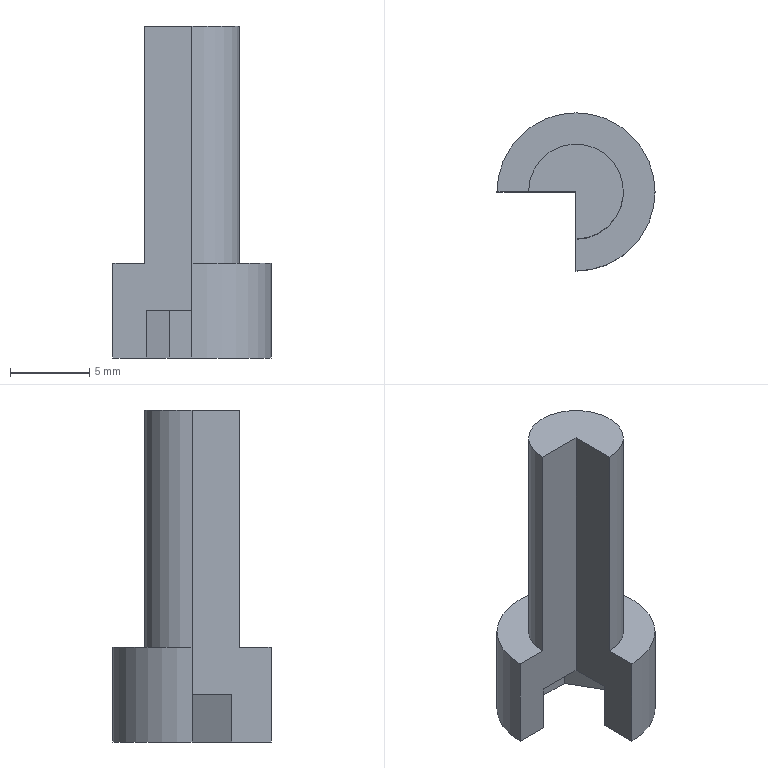Part | STEP file | LG M6_1.5F | 1 solid | 14 faces | box 10 x 10 x 21 mm | volume 622.411 mm3 | plane 11 | cylinder 3 | commonest cylinder face diameters 10 x2 6 x1
STEP:
#1=CARTESIAN_POINT('',(0.,0.,0.));
#2=DIRECTION('',(0.,0.,1.));
#3=DIRECTION('',(1.,0.,0.));
#4=AXIS2_PLACEMENT_3D('',#1,#2,#3);
#5=CARTESIAN_POINT('',(0.,-5.,-6.));
#6=VERTEX_POINT('',#5);
#7=CARTESIAN_POINT('',(5.,0.,-6.));
#8=VERTEX_POINT('',#7);
#9=CARTESIAN_POINT('',(0.,0.,-6.));
#10=DIRECTION('',(0.,0.,1.));
#11=DIRECTION('',(1.,0.,0.));
#12=AXIS2_PLACEMENT_3D('',#9,#10,#11);
#13=CIRCLE('',#12,5.);
#14=CARTESIAN_POINT('',(0.,0.,-6.));
#15=DIRECTION('',(0.,0.,1.));
#16=DIRECTION('',(1.,0.,0.));
#17=AXIS2_PLACEMENT_3D('',#14,#15,#16);
#18=CYLINDRICAL_SURFACE('',#17,5.);
#19=CARTESIAN_POINT('',(0.,0.));
#20=DIRECTION('',(1.,0.));
#21=VECTOR('',#20,1.);
#22=LINE('',#19,#21);
#23=(GEOMETRIC_REPRESENTATION_CONTEXT(2)PARAMETRIC_REPRESENTATION_CONTEXT()REPRESENTATION_CONTEXT('',''));
#24=DEFINITIONAL_REPRESENTATION('',(#22),#23);
#25=PCURVE('',#18,#24);
#26=CARTESIAN_POINT('',(0.,0.,-6.));
#27=DIRECTION('',(0.,0.,1.));
#28=DIRECTION('',(1.,0.,0.));
#29=AXIS2_PLACEMENT_3D('',#26,#27,#28);
#30=PLANE('',#29);
#31=CARTESIAN_POINT('',(0.,0.));
#32=DIRECTION('',(1.,0.));
#33=AXIS2_PLACEMENT_2D('',#31,#32);
#34=CIRCLE('',#33,5.);
#35=(GEOMETRIC_REPRESENTATION_CONTEXT(2)PARAMETRIC_REPRESENTATION_CONTEXT()REPRESENTATION_CONTEXT('',''));
#36=DEFINITIONAL_REPRESENTATION('',(#34),#35);
#37=PCURVE('',#30,#36);
#38=SURFACE_CURVE('',#13,(#25,#37),.PCURVE_S1.);
#39=EDGE_CURVE('',#6,#8,#38,.T.);
#40=ORIENTED_EDGE('',*,*,#39,.T.);
#41=CARTESIAN_POINT('',(5.,0.,0.));
#42=VERTEX_POINT('',#41);
#43=CARTESIAN_POINT('',(5.,0.,-6.));
#44=DIRECTION('',(0.,0.,1.));
#45=VECTOR('',#44,1.);
#46=LINE('',#43,#45);
#47=CARTESIAN_POINT('',(6.283,0.));
#48=DIRECTION('',(0.,1.));
#49=VECTOR('',#48,1.);
#50=LINE('',#47,#49);
#51=(GEOMETRIC_REPRESENTATION_CONTEXT(2)PARAMETRIC_REPRESENTATION_CONTEXT()REPRESENTATION_CONTEXT('',''));
#52=DEFINITIONAL_REPRESENTATION('',(#50),#51);
#53=PCURVE('',#18,#52);
#54=CARTESIAN_POINT('',(0.,0.,-6.));
#55=DIRECTION('',(0.,0.,1.));
#56=DIRECTION('',(1.,0.,0.));
#57=AXIS2_PLACEMENT_3D('',#54,#55,#56);
#58=CYLINDRICAL_SURFACE('',#57,5.);
#59=CARTESIAN_POINT('',(0.,0.));
#60=DIRECTION('',(0.,1.));
#61=VECTOR('',#60,1.);
#62=LINE('',#59,#61);
#63=(GEOMETRIC_REPRESENTATION_CONTEXT(2)PARAMETRIC_REPRESENTATION_CONTEXT()REPRESENTATION_CONTEXT('',''));
#64=DEFINITIONAL_REPRESENTATION('',(#62),#63);
#65=PCURVE('',#58,#64);
#66=SURFACE_CURVE('',#46,(#53,#65),.PCURVE_S1.);
#67=EDGE_CURVE('',#8,#42,#66,.T.);
#68=ORIENTED_EDGE('',*,*,#67,.T.);
#69=CARTESIAN_POINT('',(0.,-5.,0.));
#70=VERTEX_POINT('',#69);
#71=CARTESIAN_POINT('',(0.,0.,0.));
#72=DIRECTION('',(0.,0.,1.));
#73=DIRECTION('',(1.,0.,0.));
#74=AXIS2_PLACEMENT_3D('',#71,#72,#73);
#75=CIRCLE('',#74,5.);
#76=CARTESIAN_POINT('',(0.,6.));
#77=DIRECTION('',(1.,0.));
#78=VECTOR('',#77,1.);
#79=LINE('',#76,#78);
#80=(GEOMETRIC_REPRESENTATION_CONTEXT(2)PARAMETRIC_REPRESENTATION_CONTEXT()REPRESENTATION_CONTEXT('',''));
#81=DEFINITIONAL_REPRESENTATION('',(#79),#80);
#82=PCURVE('',#18,#81);
#83=CARTESIAN_POINT('',(0.,0.,0.));
#84=DIRECTION('',(0.,0.,1.));
#85=DIRECTION('',(1.,0.,0.));
#86=AXIS2_PLACEMENT_3D('',#83,#84,#85);
#87=PLANE('',#86);
#88=CARTESIAN_POINT('',(0.,0.));
#89=DIRECTION('',(1.,0.));
#90=AXIS2_PLACEMENT_2D('',#88,#89);
#91=CIRCLE('',#90,5.);
#92=(GEOMETRIC_REPRESENTATION_CONTEXT(2)PARAMETRIC_REPRESENTATION_CONTEXT()REPRESENTATION_CONTEXT('',''));
#93=DEFINITIONAL_REPRESENTATION('',(#91),#92);
#94=PCURVE('',#87,#93);
#95=SURFACE_CURVE('',#75,(#82,#94),.PCURVE_S1.);
#96=EDGE_CURVE('',#70,#42,#95,.T.);
#97=ORIENTED_EDGE('',*,*,#96,.F.);
#98=CARTESIAN_POINT('',(0.,-5.,-6.));
#99=DIRECTION('',(0.,0.,-1.));
#100=VECTOR('',#99,1.);
#101=LINE('',#98,#100);
#102=CARTESIAN_POINT('',(4.712,0.));
#103=DIRECTION('',(0.,-1.));
#104=VECTOR('',#103,1.);
#105=LINE('',#102,#104);
#106=(GEOMETRIC_REPRESENTATION_CONTEXT(2)PARAMETRIC_REPRESENTATION_CONTEXT()REPRESENTATION_CONTEXT('',''));
#107=DEFINITIONAL_REPRESENTATION('',(#105),#106);
#108=PCURVE('',#18,#107);
#109=CARTESIAN_POINT('',(0.,33.935,109.834));
#110=DIRECTION('',(-1.,0.,0.));
#111=DIRECTION('',(0.,1.,0.));
#112=AXIS2_PLACEMENT_3D('',#109,#110,#111);
#113=PLANE('',#112);
#114=CARTESIAN_POINT('',(-38.935,115.834));
#115=DIRECTION('',(0.,1.));
#116=VECTOR('',#115,1.);
#117=LINE('',#114,#116);
#118=(GEOMETRIC_REPRESENTATION_CONTEXT(2)PARAMETRIC_REPRESENTATION_CONTEXT()REPRESENTATION_CONTEXT('',''));
#119=DEFINITIONAL_REPRESENTATION('',(#117),#118);
#120=PCURVE('',#113,#119);
#121=SURFACE_CURVE('',#101,(#108,#120),.PCURVE_S1.);
#122=EDGE_CURVE('',#70,#6,#121,.T.);
#123=ORIENTED_EDGE('',*,*,#122,.T.);
#124=EDGE_LOOP('',(#40,#68,#97,#123));
#125=FACE_BOUND('',#124,.T.);
#126=ADVANCED_FACE('',(#125),#18,.T.);
#127=CARTESIAN_POINT('',(0.,-2.51,-3.));
#128=VERTEX_POINT('',#127);
#129=CARTESIAN_POINT('',(0.,-2.51,-6.));
#130=VERTEX_POINT('',#129);
#131=CARTESIAN_POINT('',(0.,-2.51,-3.));
#132=DIRECTION('',(0.,0.,-1.));
#133=VECTOR('',#132,1.);
#134=LINE('',#131,#133);
#135=CARTESIAN_POINT('',(1.449,-2.51,-3.));
#136=DIRECTION('',(0.,-1.,0.));
#137=DIRECTION('',(0.,0.,-1.));
#138=AXIS2_PLACEMENT_3D('',#135,#136,#137);
#139=PLANE('',#138);
#140=CARTESIAN_POINT('',(0.,-1.449));
#141=DIRECTION('',(1.,0.));
#142=VECTOR('',#141,1.);
#143=LINE('',#140,#142);
#144=(GEOMETRIC_REPRESENTATION_CONTEXT(2)PARAMETRIC_REPRESENTATION_CONTEXT()REPRESENTATION_CONTEXT('',''));
#145=DEFINITIONAL_REPRESENTATION('',(#143),#144);
#146=PCURVE('',#139,#145);
#147=CARTESIAN_POINT('',(-36.445,112.834));
#148=DIRECTION('',(0.,1.));
#149=VECTOR('',#148,1.);
#150=LINE('',#147,#149);
#151=(GEOMETRIC_REPRESENTATION_CONTEXT(2)PARAMETRIC_REPRESENTATION_CONTEXT()REPRESENTATION_CONTEXT('',''));
#152=DEFINITIONAL_REPRESENTATION('',(#150),#151);
#153=PCURVE('',#113,#152);
#154=SURFACE_CURVE('',#134,(#146,#153),.PCURVE_S1.);
#155=EDGE_CURVE('',#128,#130,#154,.T.);
#156=ORIENTED_EDGE('',*,*,#155,.F.);
#157=CARTESIAN_POINT('',(1.449,-2.51,-3.));
#158=VERTEX_POINT('',#157);
#159=CARTESIAN_POINT('',(1.449,-2.51,-3.));
#160=DIRECTION('',(-1.,0.,0.));
#161=VECTOR('',#160,1.);
#162=LINE('',#159,#161);
#163=CARTESIAN_POINT('',(0.,0.));
#164=DIRECTION('',(0.,-1.));
#165=VECTOR('',#164,1.);
#166=LINE('',#163,#165);
#167=(GEOMETRIC_REPRESENTATION_CONTEXT(2)PARAMETRIC_REPRESENTATION_CONTEXT()REPRESENTATION_CONTEXT('',''));
#168=DEFINITIONAL_REPRESENTATION('',(#166),#167);
#169=PCURVE('',#139,#168);
#170=CARTESIAN_POINT('',(0.,0.,-3.));
#171=DIRECTION('',(0.,0.,-1.));
#172=DIRECTION('',(-1.,0.,0.));
#173=AXIS2_PLACEMENT_3D('',#170,#171,#172);
#174=PLANE('',#173);
#175=CARTESIAN_POINT('',(-1.449,-2.51));
#176=DIRECTION('',(1.,0.));
#177=VECTOR('',#176,1.);
#178=LINE('',#175,#177);
#179=(GEOMETRIC_REPRESENTATION_CONTEXT(2)PARAMETRIC_REPRESENTATION_CONTEXT()REPRESENTATION_CONTEXT('',''));
#180=DEFINITIONAL_REPRESENTATION('',(#178),#179);
#181=PCURVE('',#174,#180);
#182=SURFACE_CURVE('',#162,(#169,#181),.PCURVE_S1.);
#183=EDGE_CURVE('',#158,#128,#182,.T.);
#184=ORIENTED_EDGE('',*,*,#183,.F.);
#185=CARTESIAN_POINT('',(1.449,-2.51,-6.));
#186=VERTEX_POINT('',#185);
#187=CARTESIAN_POINT('',(1.449,-2.51,-3.));
#188=DIRECTION('',(0.,0.,-1.));
#189=VECTOR('',#188,1.);
#190=LINE('',#187,#189);
#191=CARTESIAN_POINT('',(0.,0.));
#192=DIRECTION('',(1.,0.));
#193=VECTOR('',#192,1.);
#194=LINE('',#191,#193);
#195=(GEOMETRIC_REPRESENTATION_CONTEXT(2)PARAMETRIC_REPRESENTATION_CONTEXT()REPRESENTATION_CONTEXT('',''));
#196=DEFINITIONAL_REPRESENTATION('',(#194),#195);
#197=PCURVE('',#139,#196);
#198=CARTESIAN_POINT('',(2.898,0.,-3.));
#199=DIRECTION('',(0.866,-0.5,0.));
#200=DIRECTION('',(0.5,0.866,0.));
#201=AXIS2_PLACEMENT_3D('',#198,#199,#200);
#202=PLANE('',#201);
#203=CARTESIAN_POINT('',(-2.898,0.));
#204=DIRECTION('',(0.,-1.));
#205=VECTOR('',#204,1.);
#206=LINE('',#203,#205);
#207=(GEOMETRIC_REPRESENTATION_CONTEXT(2)PARAMETRIC_REPRESENTATION_CONTEXT()REPRESENTATION_CONTEXT('',''));
#208=DEFINITIONAL_REPRESENTATION('',(#206),#207);
#209=PCURVE('',#202,#208);
#210=SURFACE_CURVE('',#190,(#197,#209),.PCURVE_S1.);
#211=EDGE_CURVE('',#158,#186,#210,.T.);
#212=ORIENTED_EDGE('',*,*,#211,.T.);
#213=CARTESIAN_POINT('',(1.449,-2.51,-6.));
#214=DIRECTION('',(-1.,0.,0.));
#215=VECTOR('',#214,1.);
#216=LINE('',#213,#215);
#217=CARTESIAN_POINT('',(3.,0.));
#218=DIRECTION('',(0.,-1.));
#219=VECTOR('',#218,1.);
#220=LINE('',#217,#219);
#221=(GEOMETRIC_REPRESENTATION_CONTEXT(2)PARAMETRIC_REPRESENTATION_CONTEXT()REPRESENTATION_CONTEXT('',''));
#222=DEFINITIONAL_REPRESENTATION('',(#220),#221);
#223=PCURVE('',#139,#222);
#224=CARTESIAN_POINT('',(1.449,-2.51));
#225=DIRECTION('',(-1.,0.));
#226=VECTOR('',#225,1.);
#227=LINE('',#224,#226);
#228=(GEOMETRIC_REPRESENTATION_CONTEXT(2)PARAMETRIC_REPRESENTATION_CONTEXT()REPRESENTATION_CONTEXT('',''));
#229=DEFINITIONAL_REPRESENTATION('',(#227),#228);
#230=PCURVE('',#30,#229);
#231=SURFACE_CURVE('',#216,(#223,#230),.PCURVE_S1.);
#232=EDGE_CURVE('',#186,#130,#231,.T.);
#233=ORIENTED_EDGE('',*,*,#232,.T.);
#234=EDGE_LOOP('',(#156,#184,#212,#233));
#235=FACE_BOUND('',#234,.T.);
#236=ADVANCED_FACE('',(#235),#139,.F.);
#237=CARTESIAN_POINT('',(-3.,0.,0.));
#238=VERTEX_POINT('',#237);
#239=CARTESIAN_POINT('',(-5.,0.,0.));
#240=VERTEX_POINT('',#239);
#241=CARTESIAN_POINT('',(0.,0.,0.));
#242=DIRECTION('',(-1.,0.,0.));
#243=VECTOR('',#242,1.);
#244=LINE('',#241,#243);
#245=CARTESIAN_POINT('',(0.,0.));
#246=DIRECTION('',(-1.,0.));
#247=VECTOR('',#246,1.);
#248=LINE('',#245,#247);
#249=(GEOMETRIC_REPRESENTATION_CONTEXT(2)PARAMETRIC_REPRESENTATION_CONTEXT()REPRESENTATION_CONTEXT('',''));
#250=DEFINITIONAL_REPRESENTATION('',(#248),#249);
#251=PCURVE('',#87,#250);
#252=CARTESIAN_POINT('',(0.,0.,98.57));
#253=DIRECTION('',(0.,1.,0.));
#254=DIRECTION('',(1.,0.,0.));
#255=AXIS2_PLACEMENT_3D('',#252,#253,#254);
#256=PLANE('',#255);
#257=CARTESIAN_POINT('',(0.,98.57));
#258=DIRECTION('',(-1.,0.));
#259=VECTOR('',#258,1.);
#260=LINE('',#257,#259);
#261=(GEOMETRIC_REPRESENTATION_CONTEXT(2)PARAMETRIC_REPRESENTATION_CONTEXT()REPRESENTATION_CONTEXT('',''));
#262=DEFINITIONAL_REPRESENTATION('',(#260),#261);
#263=PCURVE('',#256,#262);
#264=SURFACE_CURVE('',#244,(#251,#263),.PCURVE_S1.);
#265=EDGE_CURVE('',#238,#240,#264,.T.);
#266=ORIENTED_EDGE('',*,*,#265,.F.);
#267=CARTESIAN_POINT('',(0.,-3.,0.));
#268=VERTEX_POINT('',#267);
#269=CARTESIAN_POINT('',(0.,0.,0.));
#270=DIRECTION('',(0.,0.,1.));
#271=DIRECTION('',(1.,0.,0.));
#272=AXIS2_PLACEMENT_3D('',#269,#270,#271);
#273=CIRCLE('',#272,3.);
#274=CARTESIAN_POINT('',(0.,0.));
#275=DIRECTION('',(1.,0.));
#276=AXIS2_PLACEMENT_2D('',#274,#275);
#277=CIRCLE('',#276,3.);
#278=(GEOMETRIC_REPRESENTATION_CONTEXT(2)PARAMETRIC_REPRESENTATION_CONTEXT()REPRESENTATION_CONTEXT('',''));
#279=DEFINITIONAL_REPRESENTATION('',(#277),#278);
#280=PCURVE('',#87,#279);
#281=CARTESIAN_POINT('',(0.,0.,15.));
#282=DIRECTION('',(0.,0.,-1.));
#283=DIRECTION('',(-1.,0.,0.));
#284=AXIS2_PLACEMENT_3D('',#281,#282,#283);
#285=CYLINDRICAL_SURFACE('',#284,3.);
#286=CARTESIAN_POINT('',(9.425,15.));
#287=DIRECTION('',(-1.,0.));
#288=VECTOR('',#287,1.);
#289=LINE('',#286,#288);
#290=(GEOMETRIC_REPRESENTATION_CONTEXT(2)PARAMETRIC_REPRESENTATION_CONTEXT()REPRESENTATION_CONTEXT('',''));
#291=DEFINITIONAL_REPRESENTATION('',(#289),#290);
#292=PCURVE('',#285,#291);
#293=SURFACE_CURVE('',#273,(#280,#292),.PCURVE_S1.);
#294=EDGE_CURVE('',#268,#238,#293,.T.);
#295=ORIENTED_EDGE('',*,*,#294,.F.);
#296=CARTESIAN_POINT('',(0.,0.,0.));
#297=DIRECTION('',(0.,-1.,0.));
#298=VECTOR('',#297,1.);
#299=LINE('',#296,#298);
#300=CARTESIAN_POINT('',(0.,0.));
#301=DIRECTION('',(0.,-1.));
#302=VECTOR('',#301,1.);
#303=LINE('',#300,#302);
#304=(GEOMETRIC_REPRESENTATION_CONTEXT(2)PARAMETRIC_REPRESENTATION_CONTEXT()REPRESENTATION_CONTEXT('',''));
#305=DEFINITIONAL_REPRESENTATION('',(#303),#304);
#306=PCURVE('',#87,#305);
#307=CARTESIAN_POINT('',(-33.935,109.834));
#308=DIRECTION('',(-1.,0.));
#309=VECTOR('',#308,1.);
#310=LINE('',#307,#309);
#311=(GEOMETRIC_REPRESENTATION_CONTEXT(2)PARAMETRIC_REPRESENTATION_CONTEXT()REPRESENTATION_CONTEXT('',''));
#312=DEFINITIONAL_REPRESENTATION('',(#310),#311);
#313=PCURVE('',#113,#312);
#314=SURFACE_CURVE('',#299,(#306,#313),.PCURVE_S1.);
#315=EDGE_CURVE('',#268,#70,#314,.T.);
#316=ORIENTED_EDGE('',*,*,#315,.T.);
#317=ORIENTED_EDGE('',*,*,#96,.T.);
#318=CARTESIAN_POINT('',(0.,0.,0.));
#319=DIRECTION('',(0.,0.,1.));
#320=DIRECTION('',(1.,0.,0.));
#321=AXIS2_PLACEMENT_3D('',#318,#319,#320);
#322=CIRCLE('',#321,5.);
#323=CARTESIAN_POINT('',(0.,0.));
#324=DIRECTION('',(1.,0.));
#325=AXIS2_PLACEMENT_2D('',#323,#324);
#326=CIRCLE('',#325,5.);
#327=(GEOMETRIC_REPRESENTATION_CONTEXT(2)PARAMETRIC_REPRESENTATION_CONTEXT()REPRESENTATION_CONTEXT('',''));
#328=DEFINITIONAL_REPRESENTATION('',(#326),#327);
#329=PCURVE('',#87,#328);
#330=CARTESIAN_POINT('',(0.,6.));
#331=DIRECTION('',(1.,0.));
#332=VECTOR('',#331,1.);
#333=LINE('',#330,#332);
#334=(GEOMETRIC_REPRESENTATION_CONTEXT(2)PARAMETRIC_REPRESENTATION_CONTEXT()REPRESENTATION_CONTEXT('',''));
#335=DEFINITIONAL_REPRESENTATION('',(#333),#334);
#336=PCURVE('',#58,#335);
#337=SURFACE_CURVE('',#322,(#329,#336),.PCURVE_S1.);
#338=EDGE_CURVE('',#42,#240,#337,.T.);
#339=ORIENTED_EDGE('',*,*,#338,.T.);
#340=EDGE_LOOP('',(#266,#295,#316,#317,#339));
#341=FACE_BOUND('',#340,.T.);
#342=ADVANCED_FACE('',(#341),#87,.T.);
#343=ORIENTED_EDGE('',*,*,#67,.F.);
#344=CARTESIAN_POINT('',(-5.,0.,-6.));
#345=VERTEX_POINT('',#344);
#346=CARTESIAN_POINT('',(0.,0.,-6.));
#347=DIRECTION('',(0.,0.,1.));
#348=DIRECTION('',(1.,0.,0.));
#349=AXIS2_PLACEMENT_3D('',#346,#347,#348);
#350=CIRCLE('',#349,5.);
#351=CARTESIAN_POINT('',(0.,0.));
#352=DIRECTION('',(1.,0.));
#353=VECTOR('',#352,1.);
#354=LINE('',#351,#353);
#355=(GEOMETRIC_REPRESENTATION_CONTEXT(2)PARAMETRIC_REPRESENTATION_CONTEXT()REPRESENTATION_CONTEXT('',''));
#356=DEFINITIONAL_REPRESENTATION('',(#354),#355);
#357=PCURVE('',#58,#356);
#358=CARTESIAN_POINT('',(0.,0.));
#359=DIRECTION('',(1.,0.));
#360=AXIS2_PLACEMENT_2D('',#358,#359);
#361=CIRCLE('',#360,5.);
#362=(GEOMETRIC_REPRESENTATION_CONTEXT(2)PARAMETRIC_REPRESENTATION_CONTEXT()REPRESENTATION_CONTEXT('',''));
#363=DEFINITIONAL_REPRESENTATION('',(#361),#362);
#364=PCURVE('',#30,#363);
#365=SURFACE_CURVE('',#350,(#357,#364),.PCURVE_S1.);
#366=EDGE_CURVE('',#8,#345,#365,.T.);
#367=ORIENTED_EDGE('',*,*,#366,.T.);
#368=CARTESIAN_POINT('',(-5.,0.,-6.));
#369=DIRECTION('',(0.,0.,-1.));
#370=VECTOR('',#369,1.);
#371=LINE('',#368,#370);
#372=CARTESIAN_POINT('',(3.142,0.));
#373=DIRECTION('',(0.,-1.));
#374=VECTOR('',#373,1.);
#375=LINE('',#372,#374);
#376=(GEOMETRIC_REPRESENTATION_CONTEXT(2)PARAMETRIC_REPRESENTATION_CONTEXT()REPRESENTATION_CONTEXT('',''));
#377=DEFINITIONAL_REPRESENTATION('',(#375),#376);
#378=PCURVE('',#58,#377);
#379=CARTESIAN_POINT('',(-5.,104.57));
#380=DIRECTION('',(0.,1.));
#381=VECTOR('',#380,1.);
#382=LINE('',#379,#381);
#383=(GEOMETRIC_REPRESENTATION_CONTEXT(2)PARAMETRIC_REPRESENTATION_CONTEXT()REPRESENTATION_CONTEXT('',''));
#384=DEFINITIONAL_REPRESENTATION('',(#382),#383);
#385=PCURVE('',#256,#384);
#386=SURFACE_CURVE('',#371,(#378,#385),.PCURVE_S1.);
#387=EDGE_CURVE('',#240,#345,#386,.T.);
#388=ORIENTED_EDGE('',*,*,#387,.F.);
#389=ORIENTED_EDGE('',*,*,#338,.F.);
#390=EDGE_LOOP('',(#343,#367,#388,#389));
#391=FACE_BOUND('',#390,.T.);
#392=ADVANCED_FACE('',(#391),#58,.T.);
#393=CARTESIAN_POINT('',(-2.898,0.,-6.));
#394=VERTEX_POINT('',#393);
#395=CARTESIAN_POINT('',(-1.449,2.51,-6.));
#396=VERTEX_POINT('',#395);
#397=CARTESIAN_POINT('',(-2.898,0.,-6.));
#398=DIRECTION('',(0.5,0.866,0.));
#399=VECTOR('',#398,1.);
#400=LINE('',#397,#399);
#401=CARTESIAN_POINT('',(-2.898,0.));
#402=DIRECTION('',(0.5,0.866));
#403=VECTOR('',#402,1.);
#404=LINE('',#401,#403);
#405=(GEOMETRIC_REPRESENTATION_CONTEXT(2)PARAMETRIC_REPRESENTATION_CONTEXT()REPRESENTATION_CONTEXT('',''));
#406=DEFINITIONAL_REPRESENTATION('',(#404),#405);
#407=PCURVE('',#30,#406);
#408=CARTESIAN_POINT('',(-2.898,0.,-3.));
#409=DIRECTION('',(-0.866,0.5,0.));
#410=DIRECTION('',(-0.5,-0.866,0.));
#411=AXIS2_PLACEMENT_3D('',#408,#409,#410);
#412=PLANE('',#411);
#413=CARTESIAN_POINT('',(0.,-3.));
#414=DIRECTION('',(-1.,0.));
#415=VECTOR('',#414,1.);
#416=LINE('',#413,#415);
#417=(GEOMETRIC_REPRESENTATION_CONTEXT(2)PARAMETRIC_REPRESENTATION_CONTEXT()REPRESENTATION_CONTEXT('',''));
#418=DEFINITIONAL_REPRESENTATION('',(#416),#417);
#419=PCURVE('',#412,#418);
#420=SURFACE_CURVE('',#400,(#407,#419),.PCURVE_S1.);
#421=EDGE_CURVE('',#394,#396,#420,.T.);
#422=ORIENTED_EDGE('',*,*,#421,.F.);
#423=CARTESIAN_POINT('',(0.,0.,-6.));
#424=DIRECTION('',(-1.,0.,0.));
#425=VECTOR('',#424,1.);
#426=LINE('',#423,#425);
#427=CARTESIAN_POINT('',(0.,0.));
#428=DIRECTION('',(-1.,0.));
#429=VECTOR('',#428,1.);
#430=LINE('',#427,#429);
#431=(GEOMETRIC_REPRESENTATION_CONTEXT(2)PARAMETRIC_REPRESENTATION_CONTEXT()REPRESENTATION_CONTEXT('',''));
#432=DEFINITIONAL_REPRESENTATION('',(#430),#431);
#433=PCURVE('',#30,#432);
#434=CARTESIAN_POINT('',(0.,104.57));
#435=DIRECTION('',(-1.,0.));
#436=VECTOR('',#435,1.);
#437=LINE('',#434,#436);
#438=(GEOMETRIC_REPRESENTATION_CONTEXT(2)PARAMETRIC_REPRESENTATION_CONTEXT()REPRESENTATION_CONTEXT('',''));
#439=DEFINITIONAL_REPRESENTATION('',(#437),#438);
#440=PCURVE('',#256,#439);
#441=SURFACE_CURVE('',#426,(#433,#440),.PCURVE_S1.);
#442=EDGE_CURVE('',#394,#345,#441,.T.);
#443=ORIENTED_EDGE('',*,*,#442,.T.);
#444=ORIENTED_EDGE('',*,*,#366,.F.);
#445=ORIENTED_EDGE('',*,*,#39,.F.);
#446=CARTESIAN_POINT('',(0.,0.,-6.));
#447=DIRECTION('',(0.,-1.,0.));
#448=VECTOR('',#447,1.);
#449=LINE('',#446,#448);
#450=CARTESIAN_POINT('',(0.,0.));
#451=DIRECTION('',(0.,-1.));
#452=VECTOR('',#451,1.);
#453=LINE('',#450,#452);
#454=(GEOMETRIC_REPRESENTATION_CONTEXT(2)PARAMETRIC_REPRESENTATION_CONTEXT()REPRESENTATION_CONTEXT('',''));
#455=DEFINITIONAL_REPRESENTATION('',(#453),#454);
#456=PCURVE('',#30,#455);
#457=CARTESIAN_POINT('',(-33.935,115.834));
#458=DIRECTION('',(-1.,0.));
#459=VECTOR('',#458,1.);
#460=LINE('',#457,#459);
#461=(GEOMETRIC_REPRESENTATION_CONTEXT(2)PARAMETRIC_REPRESENTATION_CONTEXT()REPRESENTATION_CONTEXT('',''));
#462=DEFINITIONAL_REPRESENTATION('',(#460),#461);
#463=PCURVE('',#113,#462);
#464=SURFACE_CURVE('',#449,(#456,#463),.PCURVE_S1.);
#465=EDGE_CURVE('',#130,#6,#464,.T.);
#466=ORIENTED_EDGE('',*,*,#465,.F.);
#467=ORIENTED_EDGE('',*,*,#232,.F.);
#468=CARTESIAN_POINT('',(2.898,0.,-6.));
#469=VERTEX_POINT('',#468);
#470=CARTESIAN_POINT('',(2.898,0.,-6.));
#471=DIRECTION('',(-0.5,-0.866,0.));
#472=VECTOR('',#471,1.);
#473=LINE('',#470,#472);
#474=CARTESIAN_POINT('',(2.898,0.));
#475=DIRECTION('',(-0.5,-0.866));
#476=VECTOR('',#475,1.);
#477=LINE('',#474,#476);
#478=(GEOMETRIC_REPRESENTATION_CONTEXT(2)PARAMETRIC_REPRESENTATION_CONTEXT()REPRESENTATION_CONTEXT('',''));
#479=DEFINITIONAL_REPRESENTATION('',(#477),#478);
#480=PCURVE('',#30,#479);
#481=CARTESIAN_POINT('',(0.,-3.));
#482=DIRECTION('',(-1.,0.));
#483=VECTOR('',#482,1.);
#484=LINE('',#481,#483);
#485=(GEOMETRIC_REPRESENTATION_CONTEXT(2)PARAMETRIC_REPRESENTATION_CONTEXT()REPRESENTATION_CONTEXT('',''));
#486=DEFINITIONAL_REPRESENTATION('',(#484),#485);
#487=PCURVE('',#202,#486);
#488=SURFACE_CURVE('',#473,(#480,#487),.PCURVE_S1.);
#489=EDGE_CURVE('',#469,#186,#488,.T.);
#490=ORIENTED_EDGE('',*,*,#489,.F.);
#491=CARTESIAN_POINT('',(1.449,2.51,-6.));
#492=VERTEX_POINT('',#491);
#493=CARTESIAN_POINT('',(1.449,2.51,-6.));
#494=DIRECTION('',(0.5,-0.866,0.));
#495=VECTOR('',#494,1.);
#496=LINE('',#493,#495);
#497=CARTESIAN_POINT('',(1.449,2.51));
#498=DIRECTION('',(0.5,-0.866));
#499=VECTOR('',#498,1.);
#500=LINE('',#497,#499);
#501=(GEOMETRIC_REPRESENTATION_CONTEXT(2)PARAMETRIC_REPRESENTATION_CONTEXT()REPRESENTATION_CONTEXT('',''));
#502=DEFINITIONAL_REPRESENTATION('',(#500),#501);
#503=PCURVE('',#30,#502);
#504=CARTESIAN_POINT('',(1.449,2.51,-3.));
#505=DIRECTION('',(0.866,0.5,0.));
#506=DIRECTION('',(-0.5,0.866,0.));
#507=AXIS2_PLACEMENT_3D('',#504,#505,#506);
#508=PLANE('',#507);
#509=CARTESIAN_POINT('',(0.,-3.));
#510=DIRECTION('',(-1.,0.));
#511=VECTOR('',#510,1.);
#512=LINE('',#509,#511);
#513=(GEOMETRIC_REPRESENTATION_CONTEXT(2)PARAMETRIC_REPRESENTATION_CONTEXT()REPRESENTATION_CONTEXT('',''));
#514=DEFINITIONAL_REPRESENTATION('',(#512),#513);
#515=PCURVE('',#508,#514);
#516=SURFACE_CURVE('',#496,(#503,#515),.PCURVE_S1.);
#517=EDGE_CURVE('',#492,#469,#516,.T.);
#518=ORIENTED_EDGE('',*,*,#517,.F.);
#519=CARTESIAN_POINT('',(-1.449,2.51,-6.));
#520=DIRECTION('',(1.,0.,0.));
#521=VECTOR('',#520,1.);
#522=LINE('',#519,#521);
#523=CARTESIAN_POINT('',(-1.449,2.51));
#524=DIRECTION('',(1.,0.));
#525=VECTOR('',#524,1.);
#526=LINE('',#523,#525);
#527=(GEOMETRIC_REPRESENTATION_CONTEXT(2)PARAMETRIC_REPRESENTATION_CONTEXT()REPRESENTATION_CONTEXT('',''));
#528=DEFINITIONAL_REPRESENTATION('',(#526),#527);
#529=PCURVE('',#30,#528);
#530=CARTESIAN_POINT('',(-1.449,2.51,-3.));
#531=DIRECTION('',(0.,1.,0.));
#532=DIRECTION('',(0.,0.,1.));
#533=AXIS2_PLACEMENT_3D('',#530,#531,#532);
#534=PLANE('',#533);
#535=CARTESIAN_POINT('',(-3.,0.));
#536=DIRECTION('',(0.,1.));
#537=VECTOR('',#536,1.);
#538=LINE('',#535,#537);
#539=(GEOMETRIC_REPRESENTATION_CONTEXT(2)PARAMETRIC_REPRESENTATION_CONTEXT()REPRESENTATION_CONTEXT('',''));
#540=DEFINITIONAL_REPRESENTATION('',(#538),#539);
#541=PCURVE('',#534,#540);
#542=SURFACE_CURVE('',#522,(#529,#541),.PCURVE_S1.);
#543=EDGE_CURVE('',#396,#492,#542,.T.);
#544=ORIENTED_EDGE('',*,*,#543,.F.);
#545=EDGE_LOOP('',(#422,#443,#444,#445,#466,#467,#490,#518,#544));
#546=FACE_BOUND('',#545,.T.);
#547=ADVANCED_FACE('',(#546),#30,.F.);
#548=ORIENTED_EDGE('',*,*,#294,.T.);
#549=CARTESIAN_POINT('',(-3.,0.,15.));
#550=VERTEX_POINT('',#549);
#551=CARTESIAN_POINT('',(-3.,0.,15.));
#552=DIRECTION('',(0.,0.,1.));
#553=VECTOR('',#552,1.);
#554=LINE('',#551,#553);
#555=CARTESIAN_POINT('',(0.,0.));
#556=DIRECTION('',(0.,-1.));
#557=VECTOR('',#556,1.);
#558=LINE('',#555,#557);
#559=(GEOMETRIC_REPRESENTATION_CONTEXT(2)PARAMETRIC_REPRESENTATION_CONTEXT()REPRESENTATION_CONTEXT('',''));
#560=DEFINITIONAL_REPRESENTATION('',(#558),#559);
#561=PCURVE('',#285,#560);
#562=CARTESIAN_POINT('',(-3.,83.57));
#563=DIRECTION('',(0.,-1.));
#564=VECTOR('',#563,1.);
#565=LINE('',#562,#564);
#566=(GEOMETRIC_REPRESENTATION_CONTEXT(2)PARAMETRIC_REPRESENTATION_CONTEXT()REPRESENTATION_CONTEXT('',''));
#567=DEFINITIONAL_REPRESENTATION('',(#565),#566);
#568=PCURVE('',#256,#567);
#569=SURFACE_CURVE('',#554,(#561,#568),.PCURVE_S1.);
#570=EDGE_CURVE('',#238,#550,#569,.T.);
#571=ORIENTED_EDGE('',*,*,#570,.T.);
#572=CARTESIAN_POINT('',(0.,-3.,15.));
#573=VERTEX_POINT('',#572);
#574=CARTESIAN_POINT('',(0.,0.,15.));
#575=DIRECTION('',(0.,0.,1.));
#576=DIRECTION('',(1.,0.,0.));
#577=AXIS2_PLACEMENT_3D('',#574,#575,#576);
#578=CIRCLE('',#577,3.);
#579=CARTESIAN_POINT('',(9.425,0.));
#580=DIRECTION('',(-1.,0.));
#581=VECTOR('',#580,1.);
#582=LINE('',#579,#581);
#583=(GEOMETRIC_REPRESENTATION_CONTEXT(2)PARAMETRIC_REPRESENTATION_CONTEXT()REPRESENTATION_CONTEXT('',''));
#584=DEFINITIONAL_REPRESENTATION('',(#582),#583);
#585=PCURVE('',#285,#584);
#586=CARTESIAN_POINT('',(0.,0.,15.));
#587=DIRECTION('',(0.,0.,1.));
#588=DIRECTION('',(1.,0.,0.));
#589=AXIS2_PLACEMENT_3D('',#586,#587,#588);
#590=PLANE('',#589);
#591=CARTESIAN_POINT('',(0.,0.));
#592=DIRECTION('',(1.,0.));
#593=AXIS2_PLACEMENT_2D('',#591,#592);
#594=CIRCLE('',#593,3.);
#595=(GEOMETRIC_REPRESENTATION_CONTEXT(2)PARAMETRIC_REPRESENTATION_CONTEXT()REPRESENTATION_CONTEXT('',''));
#596=DEFINITIONAL_REPRESENTATION('',(#594),#595);
#597=PCURVE('',#590,#596);
#598=SURFACE_CURVE('',#578,(#585,#597),.PCURVE_S1.);
#599=EDGE_CURVE('',#573,#550,#598,.T.);
#600=ORIENTED_EDGE('',*,*,#599,.F.);
#601=CARTESIAN_POINT('',(0.,-3.,15.));
#602=DIRECTION('',(0.,0.,1.));
#603=VECTOR('',#602,1.);
#604=LINE('',#601,#603);
#605=CARTESIAN_POINT('',(4.712,0.));
#606=DIRECTION('',(0.,-1.));
#607=VECTOR('',#606,1.);
#608=LINE('',#605,#607);
#609=(GEOMETRIC_REPRESENTATION_CONTEXT(2)PARAMETRIC_REPRESENTATION_CONTEXT()REPRESENTATION_CONTEXT('',''));
#610=DEFINITIONAL_REPRESENTATION('',(#608),#609);
#611=PCURVE('',#285,#610);
#612=CARTESIAN_POINT('',(-36.935,94.834));
#613=DIRECTION('',(0.,-1.));
#614=VECTOR('',#613,1.);
#615=LINE('',#612,#614);
#616=(GEOMETRIC_REPRESENTATION_CONTEXT(2)PARAMETRIC_REPRESENTATION_CONTEXT()REPRESENTATION_CONTEXT('',''));
#617=DEFINITIONAL_REPRESENTATION('',(#615),#616);
#618=PCURVE('',#113,#617);
#619=SURFACE_CURVE('',#604,(#611,#618),.PCURVE_S1.);
#620=EDGE_CURVE('',#268,#573,#619,.T.);
#621=ORIENTED_EDGE('',*,*,#620,.F.);
#622=EDGE_LOOP('',(#548,#571,#600,#621));
#623=FACE_BOUND('',#622,.T.);
#624=ADVANCED_FACE('',(#623),#285,.T.);
#625=CARTESIAN_POINT('',(0.,0.,15.));
#626=VERTEX_POINT('',#625);
#627=CARTESIAN_POINT('',(0.,0.,15.));
#628=DIRECTION('',(-1.,0.,0.));
#629=VECTOR('',#628,1.);
#630=LINE('',#627,#629);
#631=CARTESIAN_POINT('',(0.,0.));
#632=DIRECTION('',(-1.,0.));
#633=VECTOR('',#632,1.);
#634=LINE('',#631,#633);
#635=(GEOMETRIC_REPRESENTATION_CONTEXT(2)PARAMETRIC_REPRESENTATION_CONTEXT()REPRESENTATION_CONTEXT('',''));
#636=DEFINITIONAL_REPRESENTATION('',(#634),#635);
#637=PCURVE('',#590,#636);
#638=CARTESIAN_POINT('',(0.,83.57));
#639=DIRECTION('',(-1.,0.));
#640=VECTOR('',#639,1.);
#641=LINE('',#638,#640);
#642=(GEOMETRIC_REPRESENTATION_CONTEXT(2)PARAMETRIC_REPRESENTATION_CONTEXT()REPRESENTATION_CONTEXT('',''));
#643=DEFINITIONAL_REPRESENTATION('',(#641),#642);
#644=PCURVE('',#256,#643);
#645=SURFACE_CURVE('',#630,(#637,#644),.PCURVE_S1.);
#646=EDGE_CURVE('',#626,#550,#645,.T.);
#647=ORIENTED_EDGE('',*,*,#646,.F.);
#648=CARTESIAN_POINT('',(0.,0.,15.));
#649=DIRECTION('',(0.,-1.,0.));
#650=VECTOR('',#649,1.);
#651=LINE('',#648,#650);
#652=CARTESIAN_POINT('',(0.,0.));
#653=DIRECTION('',(0.,-1.));
#654=VECTOR('',#653,1.);
#655=LINE('',#652,#654);
#656=(GEOMETRIC_REPRESENTATION_CONTEXT(2)PARAMETRIC_REPRESENTATION_CONTEXT()REPRESENTATION_CONTEXT('',''));
#657=DEFINITIONAL_REPRESENTATION('',(#655),#656);
#658=PCURVE('',#590,#657);
#659=CARTESIAN_POINT('',(-33.935,94.834));
#660=DIRECTION('',(-1.,0.));
#661=VECTOR('',#660,1.);
#662=LINE('',#659,#661);
#663=(GEOMETRIC_REPRESENTATION_CONTEXT(2)PARAMETRIC_REPRESENTATION_CONTEXT()REPRESENTATION_CONTEXT('',''));
#664=DEFINITIONAL_REPRESENTATION('',(#662),#663);
#665=PCURVE('',#113,#664);
#666=SURFACE_CURVE('',#651,(#658,#665),.PCURVE_S1.);
#667=EDGE_CURVE('',#626,#573,#666,.T.);
#668=ORIENTED_EDGE('',*,*,#667,.T.);
#669=ORIENTED_EDGE('',*,*,#599,.T.);
#670=EDGE_LOOP('',(#647,#668,#669));
#671=FACE_BOUND('',#670,.T.);
#672=ADVANCED_FACE('',(#671),#590,.T.);
#673=ORIENTED_EDGE('',*,*,#489,.T.);
#674=ORIENTED_EDGE('',*,*,#211,.F.);
#675=CARTESIAN_POINT('',(2.898,0.,-3.));
#676=VERTEX_POINT('',#675);
#677=CARTESIAN_POINT('',(2.898,0.,-3.));
#678=DIRECTION('',(-0.5,-0.866,0.));
#679=VECTOR('',#678,1.);
#680=LINE('',#677,#679);
#681=CARTESIAN_POINT('',(0.,0.));
#682=DIRECTION('',(-1.,0.));
#683=VECTOR('',#682,1.);
#684=LINE('',#681,#683);
#685=(GEOMETRIC_REPRESENTATION_CONTEXT(2)PARAMETRIC_REPRESENTATION_CONTEXT()REPRESENTATION_CONTEXT('',''));
#686=DEFINITIONAL_REPRESENTATION('',(#684),#685);
#687=PCURVE('',#202,#686);
#688=CARTESIAN_POINT('',(-2.898,0.));
#689=DIRECTION('',(0.5,-0.866));
#690=VECTOR('',#689,1.);
#691=LINE('',#688,#690);
#692=(GEOMETRIC_REPRESENTATION_CONTEXT(2)PARAMETRIC_REPRESENTATION_CONTEXT()REPRESENTATION_CONTEXT('',''));
#693=DEFINITIONAL_REPRESENTATION('',(#691),#692);
#694=PCURVE('',#174,#693);
#695=SURFACE_CURVE('',#680,(#687,#694),.PCURVE_S1.);
#696=EDGE_CURVE('',#676,#158,#695,.T.);
#697=ORIENTED_EDGE('',*,*,#696,.F.);
#698=CARTESIAN_POINT('',(2.898,0.,-3.));
#699=DIRECTION('',(0.,0.,-1.));
#700=VECTOR('',#699,1.);
#701=LINE('',#698,#700);
#702=CARTESIAN_POINT('',(0.,0.));
#703=DIRECTION('',(0.,-1.));
#704=VECTOR('',#703,1.);
#705=LINE('',#702,#704);
#706=(GEOMETRIC_REPRESENTATION_CONTEXT(2)PARAMETRIC_REPRESENTATION_CONTEXT()REPRESENTATION_CONTEXT('',''));
#707=DEFINITIONAL_REPRESENTATION('',(#705),#706);
#708=PCURVE('',#202,#707);
#709=CARTESIAN_POINT('',(-2.898,0.));
#710=DIRECTION('',(0.,-1.));
#711=VECTOR('',#710,1.);
#712=LINE('',#709,#711);
#713=(GEOMETRIC_REPRESENTATION_CONTEXT(2)PARAMETRIC_REPRESENTATION_CONTEXT()REPRESENTATION_CONTEXT('',''));
#714=DEFINITIONAL_REPRESENTATION('',(#712),#713);
#715=PCURVE('',#508,#714);
#716=SURFACE_CURVE('',#701,(#708,#715),.PCURVE_S1.);
#717=EDGE_CURVE('',#676,#469,#716,.T.);
#718=ORIENTED_EDGE('',*,*,#717,.T.);
#719=EDGE_LOOP('',(#673,#674,#697,#718));
#720=FACE_BOUND('',#719,.T.);
#721=ADVANCED_FACE('',(#720),#202,.F.);
#722=ORIENTED_EDGE('',*,*,#517,.T.);
#723=ORIENTED_EDGE('',*,*,#717,.F.);
#724=CARTESIAN_POINT('',(1.449,2.51,-3.));
#725=VERTEX_POINT('',#724);
#726=CARTESIAN_POINT('',(1.449,2.51,-3.));
#727=DIRECTION('',(0.5,-0.866,0.));
#728=VECTOR('',#727,1.);
#729=LINE('',#726,#728);
#730=CARTESIAN_POINT('',(0.,0.));
#731=DIRECTION('',(-1.,0.));
#732=VECTOR('',#731,1.);
#733=LINE('',#730,#732);
#734=(GEOMETRIC_REPRESENTATION_CONTEXT(2)PARAMETRIC_REPRESENTATION_CONTEXT()REPRESENTATION_CONTEXT('',''));
#735=DEFINITIONAL_REPRESENTATION('',(#733),#734);
#736=PCURVE('',#508,#735);
#737=CARTESIAN_POINT('',(-1.449,2.51));
#738=DIRECTION('',(-0.5,-0.866));
#739=VECTOR('',#738,1.);
#740=LINE('',#737,#739);
#741=(GEOMETRIC_REPRESENTATION_CONTEXT(2)PARAMETRIC_REPRESENTATION_CONTEXT()REPRESENTATION_CONTEXT('',''));
#742=DEFINITIONAL_REPRESENTATION('',(#740),#741);
#743=PCURVE('',#174,#742);
#744=SURFACE_CURVE('',#729,(#736,#743),.PCURVE_S1.);
#745=EDGE_CURVE('',#725,#676,#744,.T.);
#746=ORIENTED_EDGE('',*,*,#745,.F.);
#747=CARTESIAN_POINT('',(1.449,2.51,-3.));
#748=DIRECTION('',(0.,0.,-1.));
#749=VECTOR('',#748,1.);
#750=LINE('',#747,#749);
#751=CARTESIAN_POINT('',(0.,0.));
#752=DIRECTION('',(0.,-1.));
#753=VECTOR('',#752,1.);
#754=LINE('',#751,#753);
#755=(GEOMETRIC_REPRESENTATION_CONTEXT(2)PARAMETRIC_REPRESENTATION_CONTEXT()REPRESENTATION_CONTEXT('',''));
#756=DEFINITIONAL_REPRESENTATION('',(#754),#755);
#757=PCURVE('',#508,#756);
#758=CARTESIAN_POINT('',(0.,2.898));
#759=DIRECTION('',(-1.,0.));
#760=VECTOR('',#759,1.);
#761=LINE('',#758,#760);
#762=(GEOMETRIC_REPRESENTATION_CONTEXT(2)PARAMETRIC_REPRESENTATION_CONTEXT()REPRESENTATION_CONTEXT('',''));
#763=DEFINITIONAL_REPRESENTATION('',(#761),#762);
#764=PCURVE('',#534,#763);
#765=SURFACE_CURVE('',#750,(#757,#764),.PCURVE_S1.);
#766=EDGE_CURVE('',#725,#492,#765,.T.);
#767=ORIENTED_EDGE('',*,*,#766,.T.);
#768=EDGE_LOOP('',(#722,#723,#746,#767));
#769=FACE_BOUND('',#768,.T.);
#770=ADVANCED_FACE('',(#769),#508,.F.);
#771=ORIENTED_EDGE('',*,*,#543,.T.);
#772=ORIENTED_EDGE('',*,*,#766,.F.);
#773=CARTESIAN_POINT('',(-1.449,2.51,-3.));
#774=VERTEX_POINT('',#773);
#775=CARTESIAN_POINT('',(-1.449,2.51,-3.));
#776=DIRECTION('',(1.,0.,0.));
#777=VECTOR('',#776,1.);
#778=LINE('',#775,#777);
#779=CARTESIAN_POINT('',(0.,0.));
#780=DIRECTION('',(0.,1.));
#781=VECTOR('',#780,1.);
#782=LINE('',#779,#781);
#783=(GEOMETRIC_REPRESENTATION_CONTEXT(2)PARAMETRIC_REPRESENTATION_CONTEXT()REPRESENTATION_CONTEXT('',''));
#784=DEFINITIONAL_REPRESENTATION('',(#782),#783);
#785=PCURVE('',#534,#784);
#786=CARTESIAN_POINT('',(1.449,2.51));
#787=DIRECTION('',(-1.,0.));
#788=VECTOR('',#787,1.);
#789=LINE('',#786,#788);
#790=(GEOMETRIC_REPRESENTATION_CONTEXT(2)PARAMETRIC_REPRESENTATION_CONTEXT()REPRESENTATION_CONTEXT('',''));
#791=DEFINITIONAL_REPRESENTATION('',(#789),#790);
#792=PCURVE('',#174,#791);
#793=SURFACE_CURVE('',#778,(#785,#792),.PCURVE_S1.);
#794=EDGE_CURVE('',#774,#725,#793,.T.);
#795=ORIENTED_EDGE('',*,*,#794,.F.);
#796=CARTESIAN_POINT('',(-1.449,2.51,-3.));
#797=DIRECTION('',(0.,0.,-1.));
#798=VECTOR('',#797,1.);
#799=LINE('',#796,#798);
#800=CARTESIAN_POINT('',(0.,0.));
#801=DIRECTION('',(-1.,0.));
#802=VECTOR('',#801,1.);
#803=LINE('',#800,#802);
#804=(GEOMETRIC_REPRESENTATION_CONTEXT(2)PARAMETRIC_REPRESENTATION_CONTEXT()REPRESENTATION_CONTEXT('',''));
#805=DEFINITIONAL_REPRESENTATION('',(#803),#804);
#806=PCURVE('',#534,#805);
#807=CARTESIAN_POINT('',(-2.898,0.));
#808=DIRECTION('',(0.,-1.));
#809=VECTOR('',#808,1.);
#810=LINE('',#807,#809);
#811=(GEOMETRIC_REPRESENTATION_CONTEXT(2)PARAMETRIC_REPRESENTATION_CONTEXT()REPRESENTATION_CONTEXT('',''));
#812=DEFINITIONAL_REPRESENTATION('',(#810),#811);
#813=PCURVE('',#412,#812);
#814=SURFACE_CURVE('',#799,(#806,#813),.PCURVE_S1.);
#815=EDGE_CURVE('',#774,#396,#814,.T.);
#816=ORIENTED_EDGE('',*,*,#815,.T.);
#817=EDGE_LOOP('',(#771,#772,#795,#816));
#818=FACE_BOUND('',#817,.T.);
#819=ADVANCED_FACE('',(#818),#534,.F.);
#820=ORIENTED_EDGE('',*,*,#421,.T.);
#821=ORIENTED_EDGE('',*,*,#815,.F.);
#822=CARTESIAN_POINT('',(-2.898,0.,-3.));
#823=VERTEX_POINT('',#822);
#824=CARTESIAN_POINT('',(-2.898,0.,-3.));
#825=DIRECTION('',(0.5,0.866,0.));
#826=VECTOR('',#825,1.);
#827=LINE('',#824,#826);
#828=CARTESIAN_POINT('',(0.,0.));
#829=DIRECTION('',(-1.,0.));
#830=VECTOR('',#829,1.);
#831=LINE('',#828,#830);
#832=(GEOMETRIC_REPRESENTATION_CONTEXT(2)PARAMETRIC_REPRESENTATION_CONTEXT()REPRESENTATION_CONTEXT('',''));
#833=DEFINITIONAL_REPRESENTATION('',(#831),#832);
#834=PCURVE('',#412,#833);
#835=CARTESIAN_POINT('',(2.898,0.));
#836=DIRECTION('',(-0.5,0.866));
#837=VECTOR('',#836,1.);
#838=LINE('',#835,#837);
#839=(GEOMETRIC_REPRESENTATION_CONTEXT(2)PARAMETRIC_REPRESENTATION_CONTEXT()REPRESENTATION_CONTEXT('',''));
#840=DEFINITIONAL_REPRESENTATION('',(#838),#839);
#841=PCURVE('',#174,#840);
#842=SURFACE_CURVE('',#827,(#834,#841),.PCURVE_S1.);
#843=EDGE_CURVE('',#823,#774,#842,.T.);
#844=ORIENTED_EDGE('',*,*,#843,.F.);
#845=CARTESIAN_POINT('',(-2.898,0.,-3.));
#846=DIRECTION('',(0.,0.,-1.));
#847=VECTOR('',#846,1.);
#848=LINE('',#845,#847);
#849=CARTESIAN_POINT('',(0.,0.));
#850=DIRECTION('',(0.,-1.));
#851=VECTOR('',#850,1.);
#852=LINE('',#849,#851);
#853=(GEOMETRIC_REPRESENTATION_CONTEXT(2)PARAMETRIC_REPRESENTATION_CONTEXT()REPRESENTATION_CONTEXT('',''));
#854=DEFINITIONAL_REPRESENTATION('',(#852),#853);
#855=PCURVE('',#412,#854);
#856=CARTESIAN_POINT('',(-2.898,101.57));
#857=DIRECTION('',(0.,1.));
#858=VECTOR('',#857,1.);
#859=LINE('',#856,#858);
#860=(GEOMETRIC_REPRESENTATION_CONTEXT(2)PARAMETRIC_REPRESENTATION_CONTEXT()REPRESENTATION_CONTEXT('',''));
#861=DEFINITIONAL_REPRESENTATION('',(#859),#860);
#862=PCURVE('',#256,#861);
#863=SURFACE_CURVE('',#848,(#855,#862),.PCURVE_S1.);
#864=EDGE_CURVE('',#823,#394,#863,.T.);
#865=ORIENTED_EDGE('',*,*,#864,.T.);
#866=EDGE_LOOP('',(#820,#821,#844,#865));
#867=FACE_BOUND('',#866,.T.);
#868=ADVANCED_FACE('',(#867),#412,.F.);
#869=CARTESIAN_POINT('',(0.,0.,-3.));
#870=VERTEX_POINT('',#869);
#871=CARTESIAN_POINT('',(0.,0.,-3.));
#872=DIRECTION('',(1.,0.,0.));
#873=VECTOR('',#872,1.);
#874=LINE('',#871,#873);
#875=CARTESIAN_POINT('',(0.,0.));
#876=DIRECTION('',(-1.,0.));
#877=VECTOR('',#876,1.);
#878=LINE('',#875,#877);
#879=(GEOMETRIC_REPRESENTATION_CONTEXT(2)PARAMETRIC_REPRESENTATION_CONTEXT()REPRESENTATION_CONTEXT('',''));
#880=DEFINITIONAL_REPRESENTATION('',(#878),#879);
#881=PCURVE('',#174,#880);
#882=CARTESIAN_POINT('',(0.,101.57));
#883=DIRECTION('',(1.,0.));
#884=VECTOR('',#883,1.);
#885=LINE('',#882,#884);
#886=(GEOMETRIC_REPRESENTATION_CONTEXT(2)PARAMETRIC_REPRESENTATION_CONTEXT()REPRESENTATION_CONTEXT('',''));
#887=DEFINITIONAL_REPRESENTATION('',(#885),#886);
#888=PCURVE('',#256,#887);
#889=SURFACE_CURVE('',#874,(#881,#888),.PCURVE_S1.);
#890=EDGE_CURVE('',#823,#870,#889,.T.);
#891=ORIENTED_EDGE('',*,*,#890,.F.);
#892=ORIENTED_EDGE('',*,*,#843,.T.);
#893=ORIENTED_EDGE('',*,*,#794,.T.);
#894=ORIENTED_EDGE('',*,*,#745,.T.);
#895=ORIENTED_EDGE('',*,*,#696,.T.);
#896=ORIENTED_EDGE('',*,*,#183,.T.);
#897=CARTESIAN_POINT('',(0.,0.,-3.));
#898=DIRECTION('',(0.,1.,0.));
#899=VECTOR('',#898,1.);
#900=LINE('',#897,#899);
#901=CARTESIAN_POINT('',(0.,0.));
#902=DIRECTION('',(0.,1.));
#903=VECTOR('',#902,1.);
#904=LINE('',#901,#903);
#905=(GEOMETRIC_REPRESENTATION_CONTEXT(2)PARAMETRIC_REPRESENTATION_CONTEXT()REPRESENTATION_CONTEXT('',''));
#906=DEFINITIONAL_REPRESENTATION('',(#904),#905);
#907=PCURVE('',#174,#906);
#908=CARTESIAN_POINT('',(-33.935,112.834));
#909=DIRECTION('',(1.,0.));
#910=VECTOR('',#909,1.);
#911=LINE('',#908,#910);
#912=(GEOMETRIC_REPRESENTATION_CONTEXT(2)PARAMETRIC_REPRESENTATION_CONTEXT()REPRESENTATION_CONTEXT('',''));
#913=DEFINITIONAL_REPRESENTATION('',(#911),#912);
#914=PCURVE('',#113,#913);
#915=SURFACE_CURVE('',#900,(#907,#914),.PCURVE_S1.);
#916=EDGE_CURVE('',#128,#870,#915,.T.);
#917=ORIENTED_EDGE('',*,*,#916,.T.);
#918=EDGE_LOOP('',(#891,#892,#893,#894,#895,#896,#917));
#919=FACE_BOUND('',#918,.T.);
#920=ADVANCED_FACE('',(#919),#174,.T.);
#921=ORIENTED_EDGE('',*,*,#864,.F.);
#922=ORIENTED_EDGE('',*,*,#890,.T.);
#923=CARTESIAN_POINT('',(0.,0.,98.57));
#924=DIRECTION('',(0.,0.,-1.));
#925=VECTOR('',#924,1.);
#926=LINE('',#923,#925);
#927=CARTESIAN_POINT('',(0.,0.));
#928=DIRECTION('',(0.,1.));
#929=VECTOR('',#928,1.);
#930=LINE('',#927,#929);
#931=(GEOMETRIC_REPRESENTATION_CONTEXT(2)PARAMETRIC_REPRESENTATION_CONTEXT()REPRESENTATION_CONTEXT('',''));
#932=DEFINITIONAL_REPRESENTATION('',(#930),#931);
#933=PCURVE('',#256,#932);
#934=CARTESIAN_POINT('',(-33.935,11.264));
#935=DIRECTION('',(0.,1.));
#936=VECTOR('',#935,1.);
#937=LINE('',#934,#936);
#938=(GEOMETRIC_REPRESENTATION_CONTEXT(2)PARAMETRIC_REPRESENTATION_CONTEXT()REPRESENTATION_CONTEXT('',''));
#939=DEFINITIONAL_REPRESENTATION('',(#937),#938);
#940=PCURVE('',#113,#939);
#941=SURFACE_CURVE('',#926,(#933,#940),.PCURVE_S1.);
#942=EDGE_CURVE('',#626,#870,#941,.T.);
#943=ORIENTED_EDGE('',*,*,#942,.F.);
#944=ORIENTED_EDGE('',*,*,#646,.T.);
#945=ORIENTED_EDGE('',*,*,#570,.F.);
#946=ORIENTED_EDGE('',*,*,#265,.T.);
#947=ORIENTED_EDGE('',*,*,#387,.T.);
#948=ORIENTED_EDGE('',*,*,#442,.F.);
#949=EDGE_LOOP('',(#921,#922,#943,#944,#945,#946,#947,#948));
#950=FACE_BOUND('',#949,.T.);
#951=ADVANCED_FACE('',(#950),#256,.F.);
#952=ORIENTED_EDGE('',*,*,#942,.T.);
#953=ORIENTED_EDGE('',*,*,#916,.F.);
#954=ORIENTED_EDGE('',*,*,#155,.T.);
#955=ORIENTED_EDGE('',*,*,#465,.T.);
#956=ORIENTED_EDGE('',*,*,#122,.F.);
#957=ORIENTED_EDGE('',*,*,#315,.F.);
#958=ORIENTED_EDGE('',*,*,#620,.T.);
#959=ORIENTED_EDGE('',*,*,#667,.F.);
#960=EDGE_LOOP('',(#952,#953,#954,#955,#956,#957,#958,#959));
#961=FACE_BOUND('',#960,.T.);
#962=ADVANCED_FACE('',(#961),#113,.T.);
#963=CLOSED_SHELL('',(#126,#236,#342,#392,#547,#624,#672,#721,#770,#819,#868,#920,#951,#962));
#964=MANIFOLD_SOLID_BREP('',#963);
#965=(LENGTH_UNIT()NAMED_UNIT(*)SI_UNIT(.MILLI.,.METRE.));
#966=UNCERTAINTY_MEASURE_WITH_UNIT(LENGTH_MEASURE(0.0000001),#965,'','');
#967=(NAMED_UNIT(*)PLANE_ANGLE_UNIT()SI_UNIT($,.RADIAN.));
#968=(NAMED_UNIT(*)SI_UNIT($,.STERADIAN.)SOLID_ANGLE_UNIT());
#969=(GEOMETRIC_REPRESENTATION_CONTEXT(3)GLOBAL_UNCERTAINTY_ASSIGNED_CONTEXT((#966))GLOBAL_UNIT_ASSIGNED_CONTEXT((#965,#967,#968))REPRESENTATION_CONTEXT('',''));
#970=ADVANCED_BREP_SHAPE_REPRESENTATION('',(#4,#964),#969);